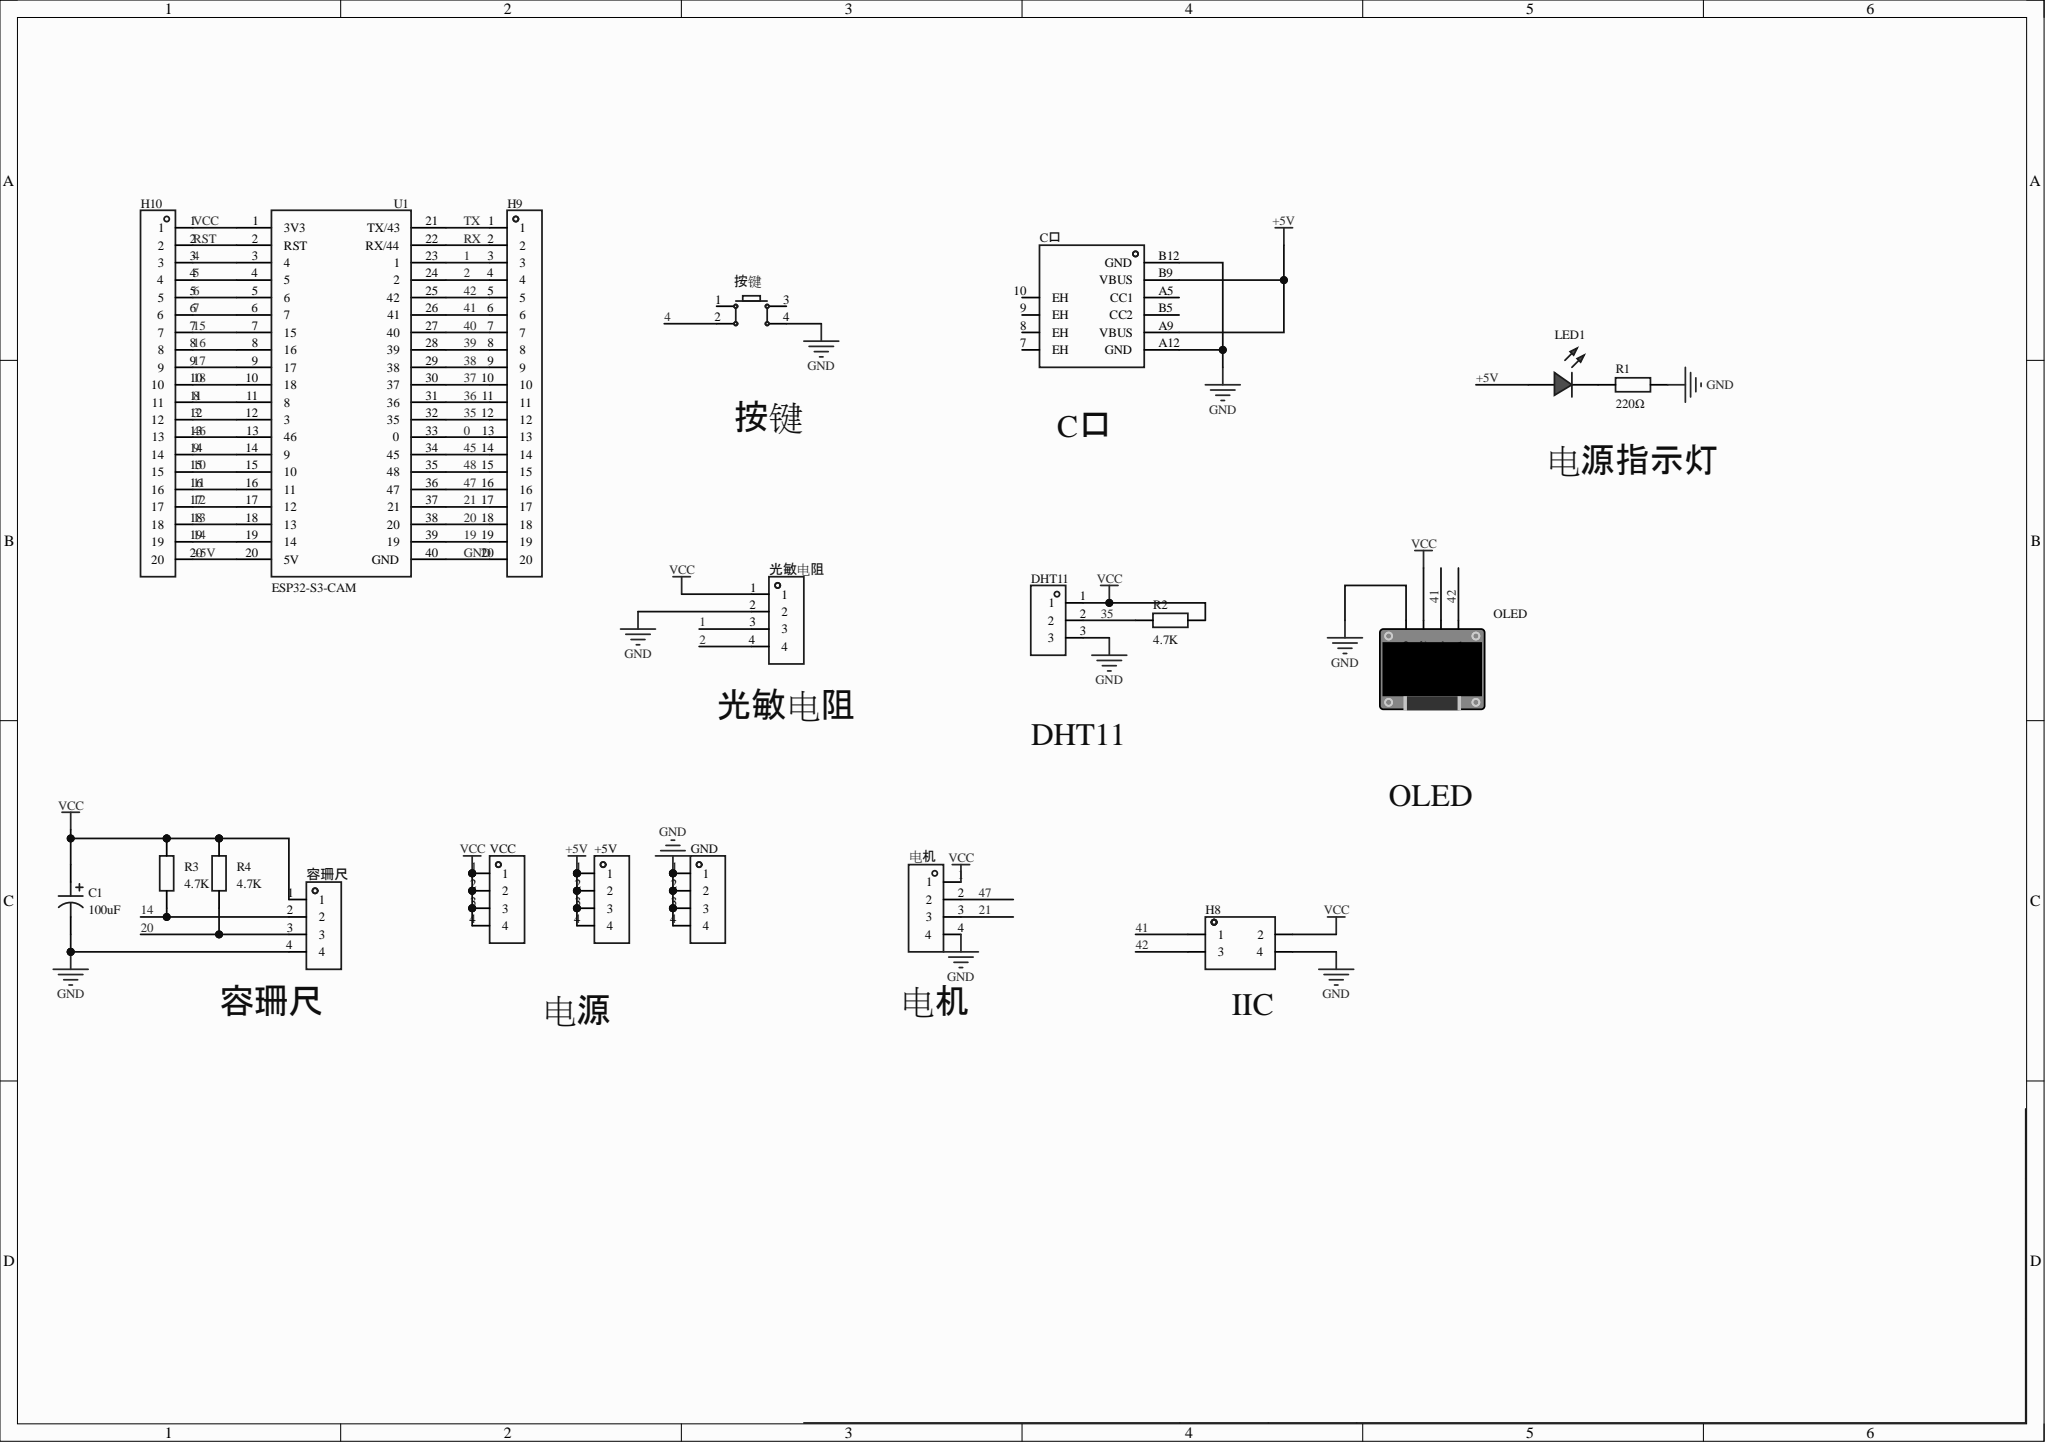Circuit board | Altium Designer | 20 parts | 41 nets
Bill of materials:
Comment,Description,Designator,Footprint,LibRef,Quantity
"","","+5V, GND, VCC, 光敏电阻, 容珊尺, 电机","HDR-TH_4P-P2.54-V-F","HDR-F_2.54_1x4P","6"
"100uF","","C1","CAP-TH_BD8.0-P3.50-D0.6-FD_1","100uF","1"
"","","C口","USB_ TYPE-C-6P","USB_ Type-C-6P","1"
"","","DHT11","HDR-TH_3P-P2.54-V-F","HDR-F_2.54_1x3P","1"
"","","H8","HDR-TH_4P-P2.54-V-F-R2-C2-S2.54","HDR-F_2.54_2x2","1"
"","间距:2.54mm;总PIN位数:20;排数:1;插针结构:-;行距:-;安装类型:直插;圆针/方针:-;额定电流:-;额定电压:-;配合针长度:-;塑高:-;触头材质:黄铜;触头镀层:-;颜色:黑色;","H9, H10","HDR-TH_20P-P2.54-V-M-1","HDR-M_2.54_1x20P","2"
"","","LED1","LED_TH-3mm","LED_TH-R_3mm","1"
"","","OLED","0.96OLED_4P","0.96OLED模块_4P","1"
"220Ω","","R1","Res_1/8W","Res_AXIAL-1/8W","1"
"4.7K","","R2, R3, R4","Res_1/8W","Res_0603","3"
"","","U1","ESP32-S3-CAM","ESP32-S3-CAM","1"
"","","按键","SW-TH_4P-L6.0-W6.0-P4.50-LS6.5","Key_TH_6x6x6","1"
Netlist (Protel format):
[
+5V
HDR-TH_4P-P2.54-V-F




]
[
C1
CAP-TH_BD8.0-P3.50-D0.6-FD_1
100uF



]
[
C口
USB_ TYPE-C-6P




]
[
DHT11
HDR-TH_3P-P2.54-V-F




]
[
GND
HDR-TH_4P-P2.54-V-F




]
[
H8
HDR-TH_4P-P2.54-V-F-R2-C2-S2.54




]
[
H9
HDR-TH_20P-P2.54-V-M-1




]
[
H10
HDR-TH_20P-P2.54-V-M-1




]
[
LED1
LED_TH-3mm




]
[
OLED
0.96OLED_4P




]
[
R1
Res_1/8W
220Ω



]
[
R2
Res_1/8W
4.7K



]
[
R3
Res_1/8W
4.7K



]
[
R4
Res_1/8W
4.7K



]
[
U1
ESP32-S3-CAM




]
[
VCC
HDR-TH_4P-P2.54-V-F




]
[
光敏电阻
HDR-TH_4P-P2.54-V-F




]
[
容珊尺
HDR-TH_4P-P2.54-V-F




]
[
按键
SW-TH_4P-L6.0-W6.0-P4.50-LS6.5




]
[
电机
HDR-TH_4P-P2.54-V-F




]
(
VCC
C1-1
DHT11-1
H8-2
H10-1
OLED-2
R2-2
R3-2
R4-2
U1-1
VCC-1
VCC-2
VCC-3
VCC-4
光敏电阻-1
容珊尺-1
电机-1
)
(
TX
H9-1
U1-21
)
(
RX
H9-2
U1-22
)
(
RST
H10-2
U1-2
)
(
NetLED1_2
LED1-2
R1-1
)
(
GND
C1-2
C口-A12
C口-B12
DHT11-3
GND-1
GND-2
GND-3
GND-4
H8-4
H9-20
OLED-1
R1-2
U1-40
光敏电阻-2
容珊尺-4
按键-4
电机-4
)
(
+5V
+5V-1
+5V-2
+5V-3
+5V-4
C口-A9
C口-B9
H10-20
LED1-1
U1-20
)
(
48
H9-15
U1-35
)
(
47
H9-16
U1-36
电机-2
)
(
46
H10-13
U1-13
)
(
45
H9-14
U1-34
)
(
42
H8-3
H9-5
OLED-4
U1-25
)
(
41
H8-1
H9-6
OLED-3
U1-26
)
(
40
H9-7
U1-27
)
(
39
H9-8
U1-28
)
(
38
H9-9
U1-29
)
(
37
H9-10
U1-30
)
(
36
H9-11
U1-31
)
(
35
DHT11-2
H9-12
R2-1
U1-32
)
(
21
H9-17
U1-37
电机-3
)
(
20
H9-18
R4-1
U1-38
容珊尺-3
)
(
19
H9-19
U1-39
)
(
18
H10-10
U1-10
)
(
17
H10-9
U1-9
)
(
16
H10-8
U1-8
)
(
15
H10-7
U1-7
)
(
14
H10-19
R3-1
U1-19
容珊尺-2
)
(
13
H10-18
U1-18
)
(
12
H10-17
U1-17
)
(
11
H10-16
U1-16
)
(
10
H10-15
U1-15
)
(
9
H10-14
U1-14
)
(
8
H10-11
U1-11
)
(
7
H10-6
U1-6
)
(
6
H10-5
U1-5
)
(
5
H10-4
U1-4
)
(
4
H10-3
U1-3
按键-2
)
(
3
H10-12
U1-12
)
(
2
H9-4
U1-24
光敏电阻-4
)
(
1
H9-3
U1-23
光敏电阻-3
)
(
0
H9-13
U1-33
)